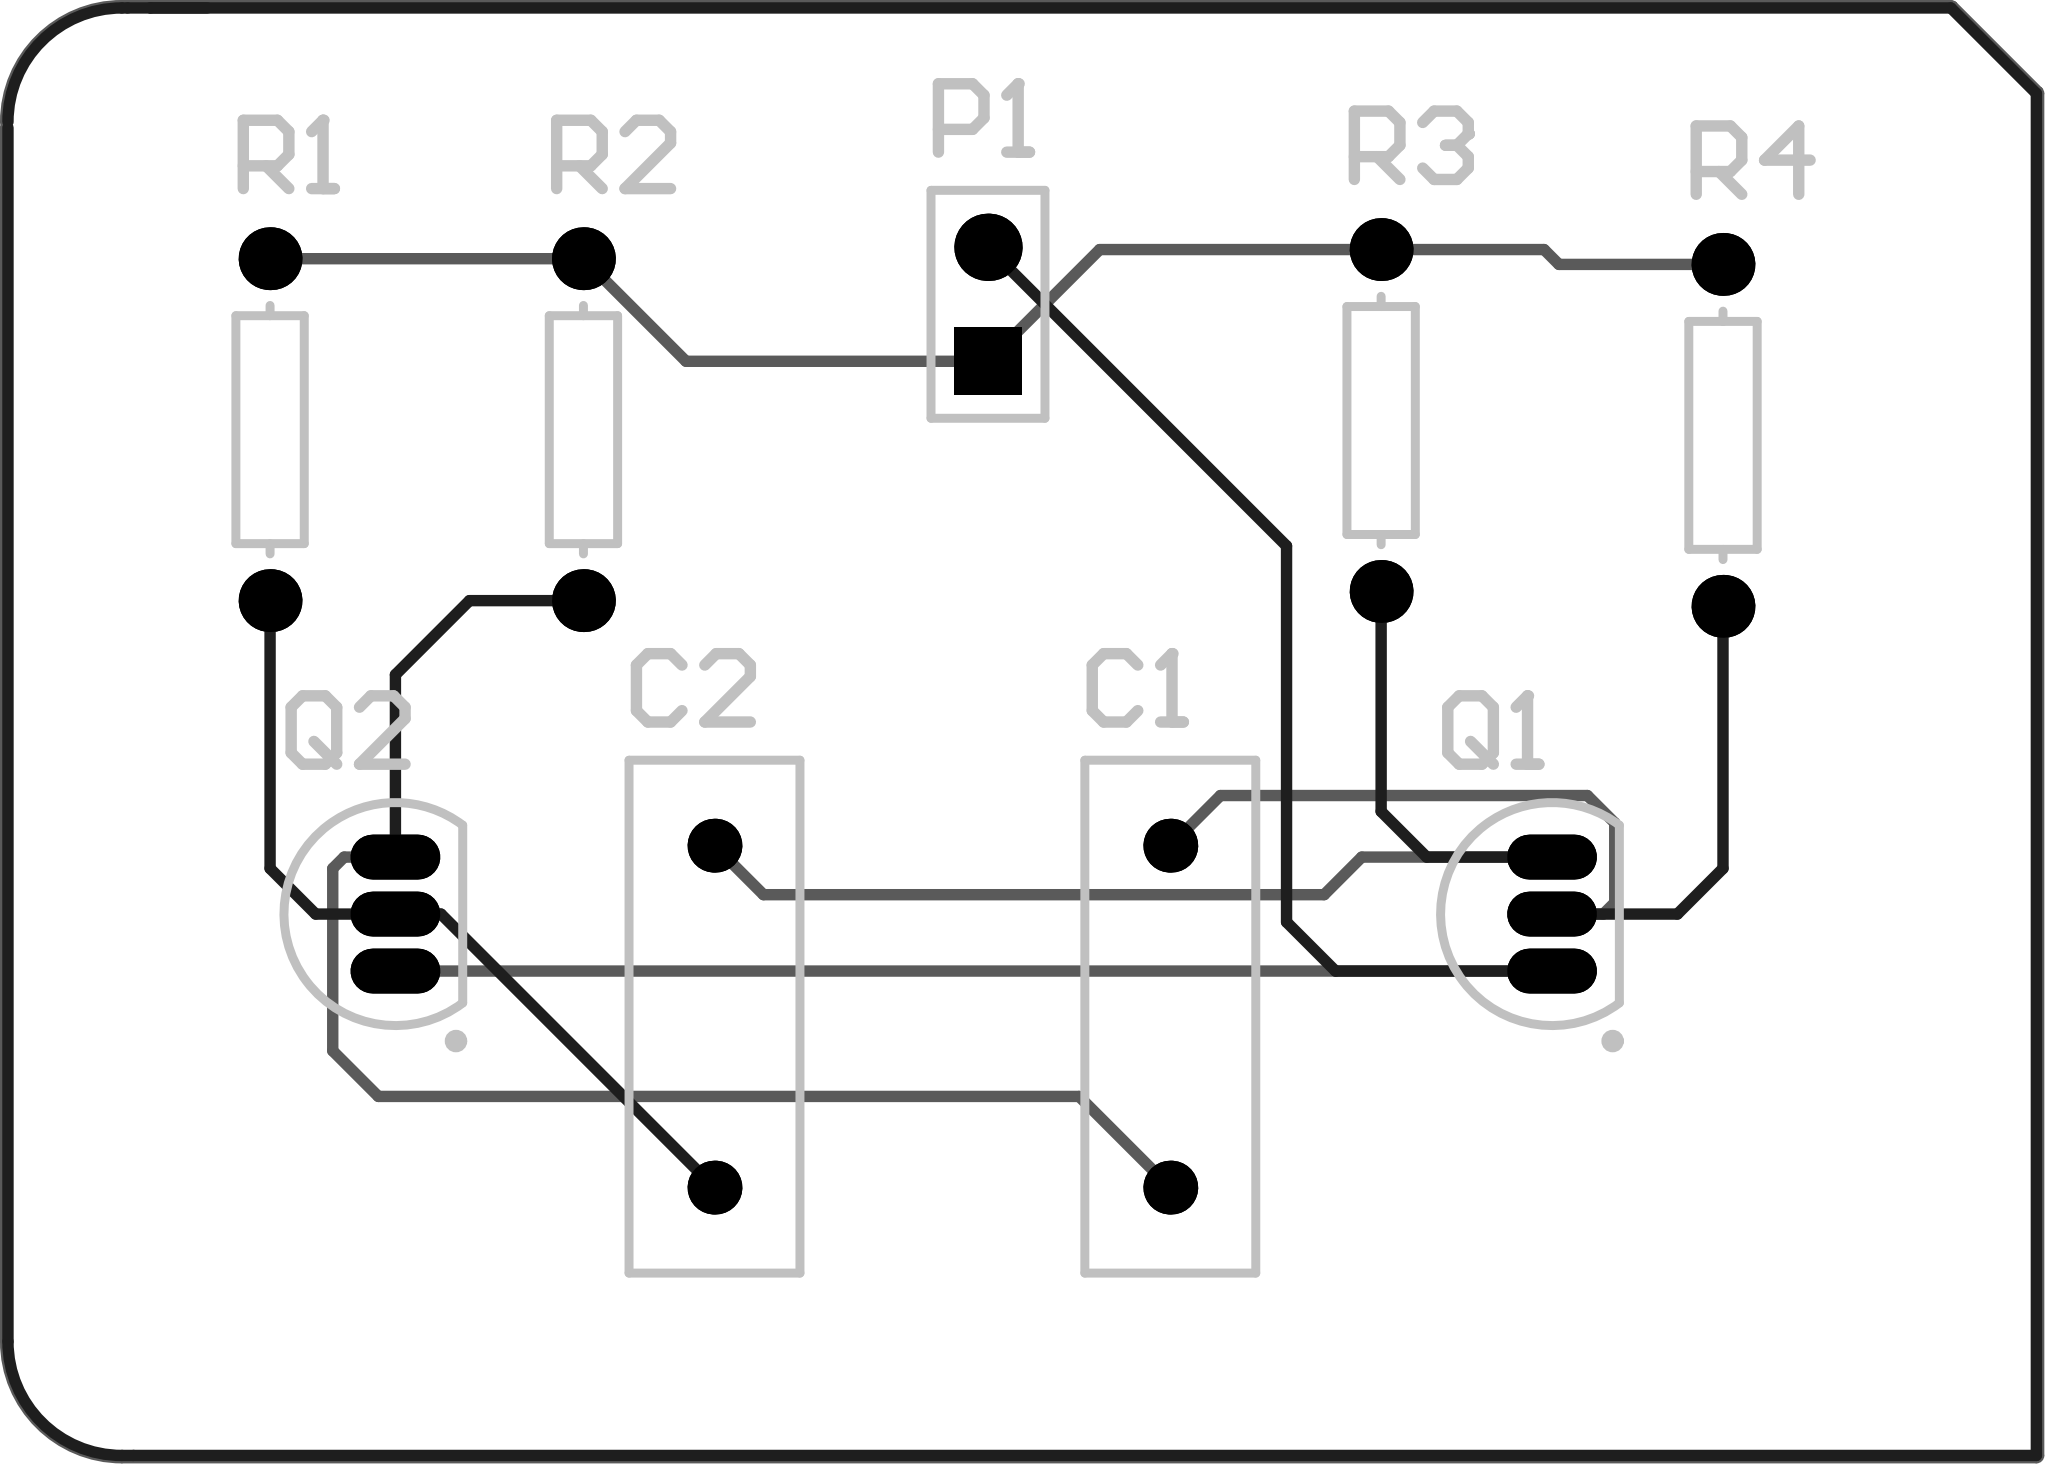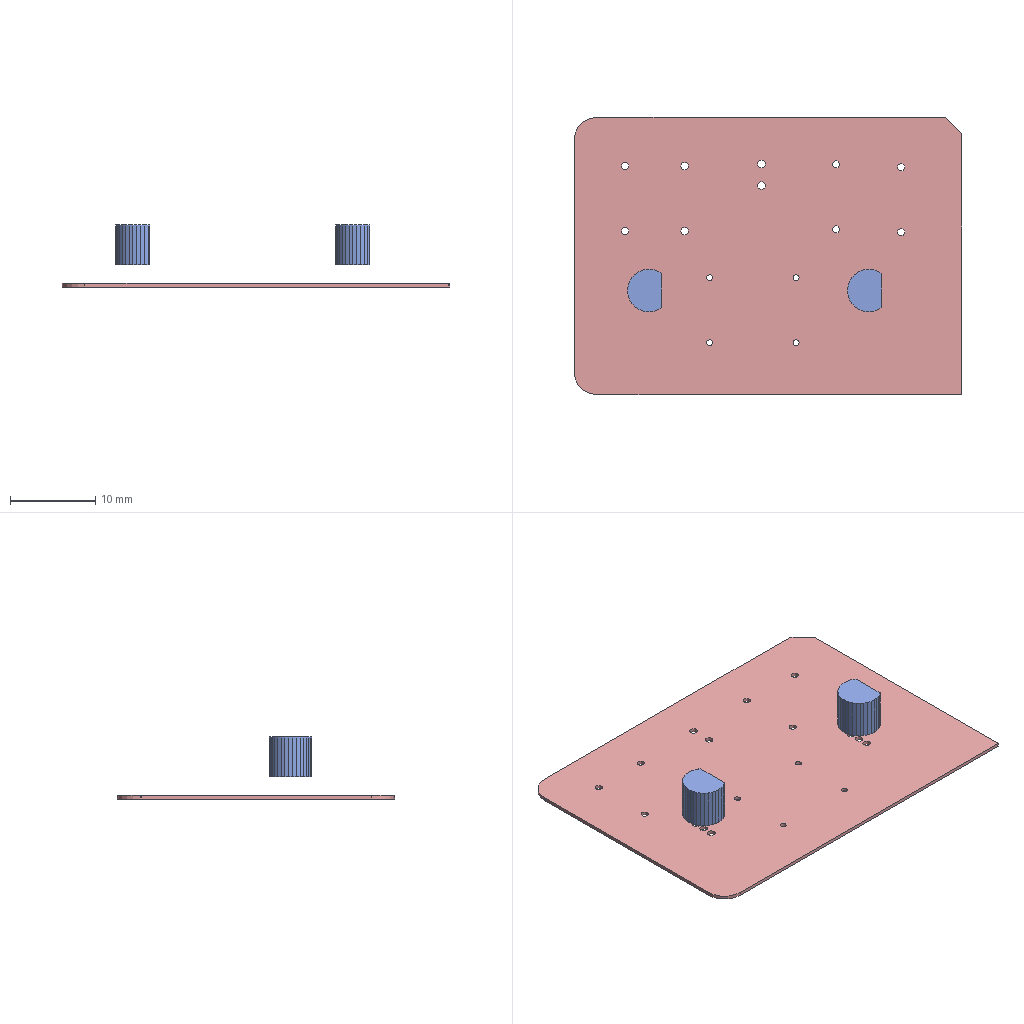Circuit board layout | Altium Designer | box 45.5 x 32.5 x 7.3 mm
Layer stack:
# Altium Designer layer stack of 4 (unit mm; dielectric type: 0 none, 1 core, 2 prepreg, 3 surface material)
index,name,kind,layer,copper_thickness_mm,dielectric_type,dielectric_thickness_mm,dielectric_material,dielectric_constant
0,Top Paste,other,,,,,,
1,Top Overlay,other,,,,,,
2,Top Solder,dielectric,,,3,0.0102,Solder Resist,3.5
3,Top Layer,copper,Top Layer,0.0356,,,,
4,Dielectric 1,dielectric,,,0,0.32,FR-4,4.8
5,Bottom Layer,copper,Bottom Layer,0.0356,,,,
6,Bottom Solder,dielectric,,,3,0.0102,Solder Resist,3.5
7,Bottom Overlay,other,,,,,,
8,Bottom Paste,other,,,,,,
# drill layer pairs: low layer,high layer
drill_pair,Top Layer,Bottom Layer
Part placement:
Designator,Comment,Layer,Footprint,Center-X(mm),Center-Y(mm),Rotation
R4,Res1,TopLayer,AXIAL-0.3,119.507,88.138,90
R3,Res1,TopLayer,AXIAL-0.3,111.887,88.469,90
R2,Res1,TopLayer,AXIAL-0.3,94.107,88.265,90
R1,Res1,TopLayer,AXIAL-0.3,87.122,88.265,90
Q2,2N3904,TopLayer,TO-92A,89.916,77.47,0
Q1,2N3904,TopLayer,TO-92A,115.697,77.47,0
P1,Header 2,TopLayer,HDR1X2,103.124,91.059,90
C2,Cap,TopLayer,RAD-0.3,97.028,75.184,90
C1,Cap,TopLayer,RAD-0.3,107.188,75.184,90
Pad and via stacks:
# Altium Designer via and pad stacks of 4 (unit mm). Each distinct definition once, with the count of objects using it.
# via: kind,start_layer,end_layer,hole_mm,diameter_mm,mode(0 simple;1 top-mid-bottom;2 full stack),diameter_per_layer,count,example_net
# pad: kind,layer,hole_mm,hole_type(0 round;1 square;2 slot),plating,top_size,top_shape(1 round;2 rect;3 octagon;9 rounded rect),mid_size,bottom_size,mode,footprint,size_per_layer,count,example
pad,Multi-Layer,0.85,0,plated,1.4x1.4,1,1.4x1.4,1.4x1.4,0,AXIAL-0.4,,14,R15.1
pad,Multi-Layer,0.7,0,plated,1.2x1.2,1,1.2x1.2,1.2x1.2,0,RAD-0.3,,4,C10.2
pad,Multi-Layer,1.6,0,plated,2.3x2.3,1,2.3x2.3,2.3x2.3,0,TO-247AC,,4,Q3.3
pad,Multi-Layer,1.6,0,plated,2.3x2.3,2,2.3x2.3,2.3x2.3,0,TO-247AC,,2,Q3.1
pad,Multi-Layer,1,0,plated,1.6x1.6,2,1.6x1.6,1.6x1.6,0,TO-220_A,,1,Q4.1
pad,Multi-Layer,1,0,plated,1.6x1.6,1,1.6x1.6,1.6x1.6,0,TO-220_A,,1,Q4.3
pad,Multi-Layer,1.27,0,plated,1.778x1.778,1,1.778x1.778,1.778x1.778,0,LED-0,,2,D1.1
pad,Top Layer,0,0,plated,0.6x2.2,1,0.6x2.2,0.6x2.2,0,M16A_N,,16,U1.1
via,Top Layer,Bottom Layer,0.7112,1.27,0,,2,NetR21_1
Design rules, without the lines most boards share:
# Altium Designer design rules of 4 (exported by Altium Designer, unit mm)
# columns: name | kind | enabled | priority | scope1 | scope2 | descriptor | typed fields (field=value)
HoleToHoleClearance | 52 | enabled | 1 | All | All | Hole To Hole Clearance (Gap=10mil) (All),(All) | gap=0.254
DiffPairsRouting | 51 | enabled | 1 | All | All | Differential Pairs Uncoupled Length using the Gap Constraints (Min=10mil) (Max=10mil) (Prefered=10mil)  and Width Constraints (Min=15mil) (Max=15mil) (Prefered=15mil) (All) |
SolderMaskExpansion | 13 | enabled | 1 | All | All | Solder Mask Expansion (Expansion =4mil) (All) | expansion=0.1016
RoutingVias | 11 | enabled | 1 | All | All | Routing Via (MinHoleWidth=28mil) (MaxHoleWidth=28mil) (PreferredHoleWidth=28mil) (MinWidth=50mil) (MaxWidth=50mil) (PreferedWidth=50mil) (All) | via_min_hole=0.7112 via_max_hole=0.7112 via_preferred_diameter=1.27 via_preferred_hole=0.7112
Width | 2 | enabled | 1 | All | All | Width Constraint (Min=10mil) (Max=10mil) (Preferred=10mil) (All) |
PolygonConnect | 20 | enabled | 1 | All | All | Polygon Connect Rule(Relief Connect )(Conductor Width=10mil) (Relief Angle=90 Angle) (Entries=4) (Air Gap Width=10mil) (All),(All) | connect_style(0=relief,1=direct,2=none)=0 relief_conductor_width=0.254 relief_entries=4
PlaneConnect | 6 | enabled | 1 | All | All | Power Plane Connect Rule(Relief Connect )(Expansion=20mil) (Conductor Width=10mil) (Air Gap=10mil) (Entries=4) (All) | relief_conductor_width=0.254 relief_entries=4 relief_expansion=0.508
Clearance | 0 | enabled | 1 | All | All | Clearance Constraint (Gap=10mil) (All),(All) | gap=0.254
Classes set for this board:
# Altium Designer classes of 4 (member kind: 0 net, 1 component, 2 from-to, 3 pad, 4 layer, 5 differential pair, 6 design channel, 7 polygon, 8 structure, 9 xSignal)
# columns: class name | member kind | superclass | members
Sheet2 | 1 | no | C10; C11; D1; Q3; Q4; Q5; R15; R16; R17; R18; R19; R20; R21; U1;
Sheet1 | 1 | no |